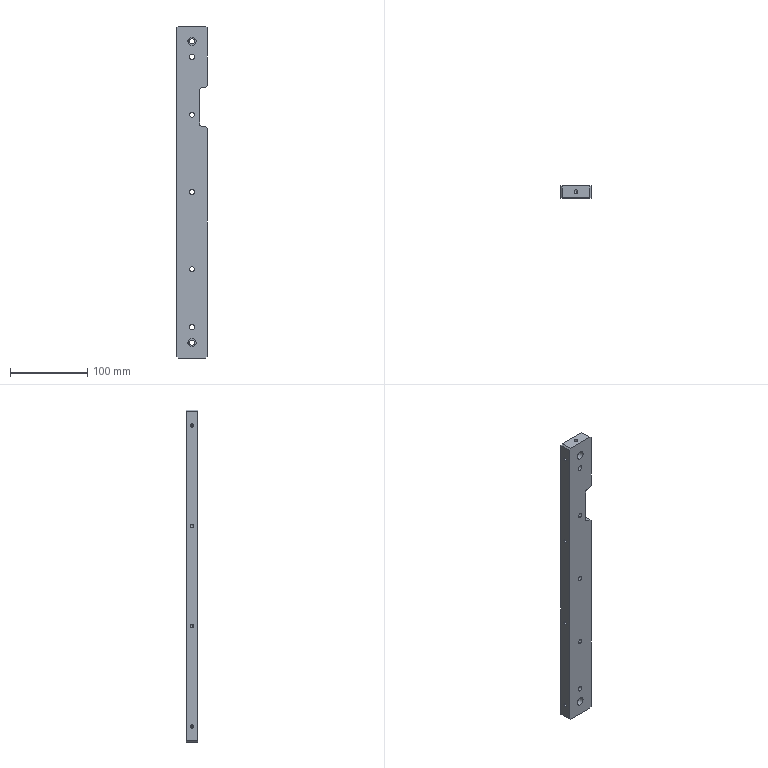Part | SolidWorks | features HoleWzd 6, Chamfer 2, ICE 2, Extrusion 1, Fillet 1 | 1 solid | 77 faces | box 40 x 15 x 430 mm | volume 242851 mm3 | cylinder 42 | plane 23 | cone 12 | commonest cylinder face diameters 6.6 x10 11 x10 4.2 x8 6 x6 5 x4 13 x4